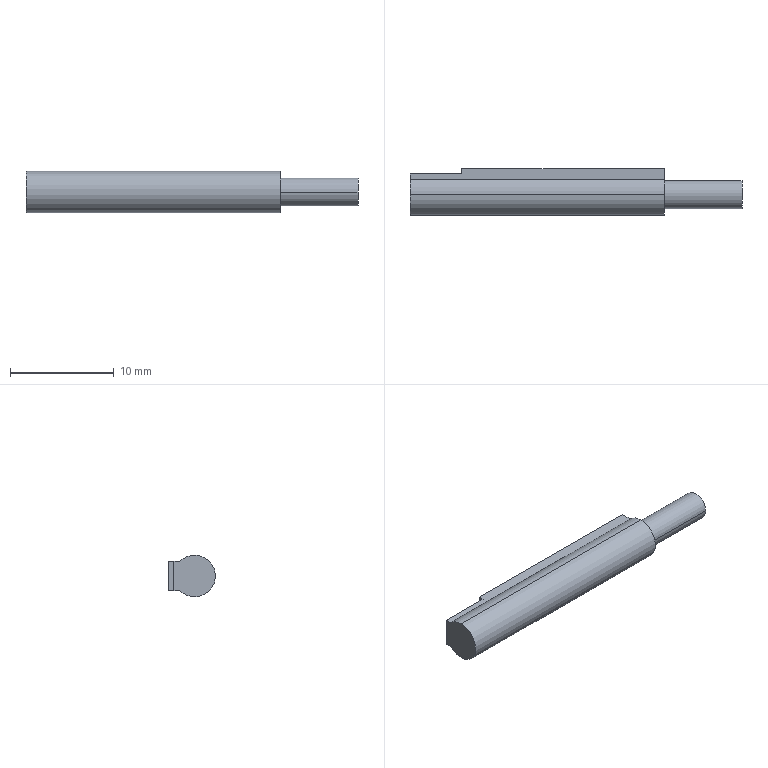Part | STEP file | 1105WWT3 | 1 solid | 16 faces | box 32 x 4.5 x 4 mm | volume 389.357 mm3 | plane 9 | cylinder 7 | commonest cylinder face diameters 4 x3 2.5 x2 2.7 x2
STEP:
#1=CARTESIAN_POINT('',(36.5,24.428,9.6));
#2=VERTEX_POINT('',#1);
#3=CARTESIAN_POINT('',(36.5,23.,9.));
#4=VERTEX_POINT('',#3);
#5=CARTESIAN_POINT('',(36.5,23.,11.));
#6=DIRECTION('',(-1.,0.,0.));
#7=DIRECTION('',(0.,0.,1.));
#8=AXIS2_PLACEMENT_3D('',#5,#6,#7);
#9=CIRCLE('',#8,2.);
#10=EDGE_CURVE('',#2,#4,#9,.T.);
#11=ORIENTED_EDGE('',*,*,#10,.T.);
#12=CARTESIAN_POINT('',(12.,23.,9.));
#13=VERTEX_POINT('',#12);
#14=CARTESIAN_POINT('',(12.,23.,9.));
#15=DIRECTION('',(-1.,0.,0.));
#16=VECTOR('',#15,1000.);
#17=LINE('',#14,#16);
#18=EDGE_CURVE('',#4,#13,#17,.T.);
#19=ORIENTED_EDGE('',*,*,#18,.T.);
#20=CARTESIAN_POINT('',(12.,24.428,9.6));
#21=VERTEX_POINT('',#20);
#22=CARTESIAN_POINT('',(12.,23.,11.));
#23=DIRECTION('',(1.,0.,0.));
#24=DIRECTION('',(0.,0.,1.));
#25=AXIS2_PLACEMENT_3D('',#22,#23,#24);
#26=CIRCLE('',#25,2.);
#27=EDGE_CURVE('',#13,#21,#26,.T.);
#28=ORIENTED_EDGE('',*,*,#27,.T.);
#29=CARTESIAN_POINT('',(12.,24.428,9.6));
#30=DIRECTION('',(1.,0.,0.));
#31=VECTOR('',#30,1000.);
#32=LINE('',#29,#31);
#33=EDGE_CURVE('',#21,#2,#32,.T.);
#34=ORIENTED_EDGE('',*,*,#33,.T.);
#35=EDGE_LOOP('',(#11,#19,#28,#34));
#36=FACE_OUTER_BOUND('',#35,.T.);
#37=CARTESIAN_POINT('',(12.,23.,11.));
#38=DIRECTION('',(-1.,0.,0.));
#39=DIRECTION('',(0.,0.,1.));
#40=AXIS2_PLACEMENT_3D('',#37,#38,#39);
#41=CYLINDRICAL_SURFACE('',#40,2.);
#42=ADVANCED_FACE('',(#36),#41,.T.);
#43=ORIENTED_EDGE('',*,*,#18,.F.);
#44=CARTESIAN_POINT('',(36.5,23.,13.));
#45=VERTEX_POINT('',#44);
#46=CARTESIAN_POINT('',(36.5,23.,11.));
#47=DIRECTION('',(-1.,0.,0.));
#48=DIRECTION('',(0.,0.,1.));
#49=AXIS2_PLACEMENT_3D('',#46,#47,#48);
#50=CIRCLE('',#49,2.);
#51=EDGE_CURVE('',#4,#45,#50,.T.);
#52=ORIENTED_EDGE('',*,*,#51,.T.);
#53=CARTESIAN_POINT('',(12.,23.,13.));
#54=VERTEX_POINT('',#53);
#55=CARTESIAN_POINT('',(12.,23.,13.));
#56=DIRECTION('',(-1.,0.,0.));
#57=VECTOR('',#56,1000.);
#58=LINE('',#55,#57);
#59=EDGE_CURVE('',#45,#54,#58,.T.);
#60=ORIENTED_EDGE('',*,*,#59,.T.);
#61=CARTESIAN_POINT('',(12.,23.,11.));
#62=DIRECTION('',(1.,0.,0.));
#63=DIRECTION('',(0.,0.,1.));
#64=AXIS2_PLACEMENT_3D('',#61,#62,#63);
#65=CIRCLE('',#64,2.);
#66=EDGE_CURVE('',#54,#13,#65,.T.);
#67=ORIENTED_EDGE('',*,*,#66,.T.);
#68=EDGE_LOOP('',(#43,#52,#60,#67));
#69=FACE_OUTER_BOUND('',#68,.T.);
#70=CARTESIAN_POINT('',(12.,23.,11.));
#71=DIRECTION('',(-1.,0.,0.));
#72=DIRECTION('',(0.,0.,1.));
#73=AXIS2_PLACEMENT_3D('',#70,#71,#72);
#74=CYLINDRICAL_SURFACE('',#73,2.);
#75=ADVANCED_FACE('',(#69),#74,.T.);
#76=CARTESIAN_POINT('',(36.5,21.65,11.));
#77=VERTEX_POINT('',#76);
#78=CARTESIAN_POINT('',(36.5,24.35,11.));
#79=VERTEX_POINT('',#78);
#80=CARTESIAN_POINT('',(36.5,23.,11.));
#81=DIRECTION('',(-1.,0.,0.));
#82=DIRECTION('',(0.,1.,0.));
#83=AXIS2_PLACEMENT_3D('',#80,#81,#82);
#84=CIRCLE('',#83,1.35);
#85=EDGE_CURVE('',#77,#79,#84,.T.);
#86=ORIENTED_EDGE('',*,*,#85,.F.);
#87=CARTESIAN_POINT('',(44.,21.65,11.));
#88=VERTEX_POINT('',#87);
#89=CARTESIAN_POINT('',(39.,21.65,11.));
#90=DIRECTION('',(1.,0.,0.));
#91=VECTOR('',#90,1000.);
#92=LINE('',#89,#91);
#93=EDGE_CURVE('',#77,#88,#92,.T.);
#94=ORIENTED_EDGE('',*,*,#93,.T.);
#95=CARTESIAN_POINT('',(44.,24.35,11.));
#96=VERTEX_POINT('',#95);
#97=CARTESIAN_POINT('',(44.,23.,11.));
#98=DIRECTION('',(-1.,0.,0.));
#99=DIRECTION('',(0.,1.,0.));
#100=AXIS2_PLACEMENT_3D('',#97,#98,#99);
#101=CIRCLE('',#100,1.35);
#102=EDGE_CURVE('',#88,#96,#101,.T.);
#103=ORIENTED_EDGE('',*,*,#102,.T.);
#104=CARTESIAN_POINT('',(39.,24.35,11.));
#105=DIRECTION('',(1.,0.,0.));
#106=VECTOR('',#105,1000.);
#107=LINE('',#104,#106);
#108=EDGE_CURVE('',#79,#96,#107,.T.);
#109=ORIENTED_EDGE('',*,*,#108,.F.);
#110=EDGE_LOOP('',(#86,#94,#103,#109));
#111=FACE_OUTER_BOUND('',#110,.T.);
#112=CARTESIAN_POINT('',(39.,23.,11.));
#113=DIRECTION('',(1.,0.,0.));
#114=DIRECTION('',(0.,1.,0.));
#115=AXIS2_PLACEMENT_3D('',#112,#113,#114);
#116=CYLINDRICAL_SURFACE('',#115,1.35);
#117=ADVANCED_FACE('',(#111),#116,.T.);
#118=CARTESIAN_POINT('',(14.,24.8,9.75));
#119=VERTEX_POINT('',#118);
#120=CARTESIAN_POINT('',(14.,24.8,12.25));
#121=VERTEX_POINT('',#120);
#122=CARTESIAN_POINT('',(14.,24.8,11.));
#123=DIRECTION('',(0.,1.,0.));
#124=DIRECTION('',(0.,0.,1.));
#125=AXIS2_PLACEMENT_3D('',#122,#123,#124);
#126=CIRCLE('',#125,1.25);
#127=EDGE_CURVE('',#119,#121,#126,.T.);
#128=ORIENTED_EDGE('',*,*,#127,.F.);
#129=CARTESIAN_POINT('',(14.,25.,9.75));
#130=VERTEX_POINT('',#129);
#131=CARTESIAN_POINT('',(14.,25.,9.75));
#132=DIRECTION('',(0.,1.,0.));
#133=VECTOR('',#132,1000.);
#134=LINE('',#131,#133);
#135=EDGE_CURVE('',#119,#130,#134,.T.);
#136=ORIENTED_EDGE('',*,*,#135,.T.);
#137=CARTESIAN_POINT('',(14.,25.,12.25));
#138=VERTEX_POINT('',#137);
#139=CARTESIAN_POINT('',(14.,25.,11.));
#140=DIRECTION('',(0.,1.,0.));
#141=DIRECTION('',(0.,0.,1.));
#142=AXIS2_PLACEMENT_3D('',#139,#140,#141);
#143=CIRCLE('',#142,1.25);
#144=EDGE_CURVE('',#130,#138,#143,.T.);
#145=ORIENTED_EDGE('',*,*,#144,.T.);
#146=CARTESIAN_POINT('',(14.,25.,12.25));
#147=DIRECTION('',(0.,1.,0.));
#148=VECTOR('',#147,1000.);
#149=LINE('',#146,#148);
#150=EDGE_CURVE('',#121,#138,#149,.T.);
#151=ORIENTED_EDGE('',*,*,#150,.F.);
#152=EDGE_LOOP('',(#128,#136,#145,#151));
#153=FACE_OUTER_BOUND('',#152,.T.);
#154=CARTESIAN_POINT('',(14.,25.,11.));
#155=DIRECTION('',(0.,1.,0.));
#156=DIRECTION('',(0.,0.,1.));
#157=AXIS2_PLACEMENT_3D('',#154,#155,#156);
#158=CYLINDRICAL_SURFACE('',#157,1.25);
#159=ADVANCED_FACE('',(#153),#158,.F.);
#160=ORIENTED_EDGE('',*,*,#59,.F.);
#161=CARTESIAN_POINT('',(36.5,24.428,12.4));
#162=VERTEX_POINT('',#161);
#163=CARTESIAN_POINT('',(36.5,23.,11.));
#164=DIRECTION('',(-1.,0.,0.));
#165=DIRECTION('',(0.,0.,1.));
#166=AXIS2_PLACEMENT_3D('',#163,#164,#165);
#167=CIRCLE('',#166,2.);
#168=EDGE_CURVE('',#45,#162,#167,.T.);
#169=ORIENTED_EDGE('',*,*,#168,.T.);
#170=CARTESIAN_POINT('',(12.,24.428,12.4));
#171=VERTEX_POINT('',#170);
#172=CARTESIAN_POINT('',(12.,24.428,12.4));
#173=DIRECTION('',(-1.,0.,0.));
#174=VECTOR('',#173,1000.);
#175=LINE('',#172,#174);
#176=EDGE_CURVE('',#162,#171,#175,.T.);
#177=ORIENTED_EDGE('',*,*,#176,.T.);
#178=CARTESIAN_POINT('',(12.,23.,11.));
#179=DIRECTION('',(1.,0.,0.));
#180=DIRECTION('',(0.,0.,1.));
#181=AXIS2_PLACEMENT_3D('',#178,#179,#180);
#182=CIRCLE('',#181,2.);
#183=EDGE_CURVE('',#171,#54,#182,.T.);
#184=ORIENTED_EDGE('',*,*,#183,.T.);
#185=EDGE_LOOP('',(#160,#169,#177,#184));
#186=FACE_OUTER_BOUND('',#185,.T.);
#187=CARTESIAN_POINT('',(12.,23.,11.));
#188=DIRECTION('',(-1.,0.,0.));
#189=DIRECTION('',(0.,0.,1.));
#190=AXIS2_PLACEMENT_3D('',#187,#188,#189);
#191=CYLINDRICAL_SURFACE('',#190,2.);
#192=ADVANCED_FACE('',(#186),#191,.T.);
#193=CARTESIAN_POINT('',(12.,25.,9.6));
#194=VERTEX_POINT('',#193);
#195=CARTESIAN_POINT('',(12.,25.5,9.6));
#196=DIRECTION('',(0.,1.,0.));
#197=VECTOR('',#196,1000.);
#198=LINE('',#195,#197);
#199=EDGE_CURVE('',#21,#194,#198,.T.);
#200=ORIENTED_EDGE('',*,*,#199,.F.);
#201=ORIENTED_EDGE('',*,*,#27,.F.);
#202=ORIENTED_EDGE('',*,*,#66,.F.);
#203=ORIENTED_EDGE('',*,*,#183,.F.);
#204=CARTESIAN_POINT('',(12.,25.,12.4));
#205=VERTEX_POINT('',#204);
#206=CARTESIAN_POINT('',(12.,23.,12.4));
#207=DIRECTION('',(0.,-1.,0.));
#208=VECTOR('',#207,1000.);
#209=LINE('',#206,#208);
#210=EDGE_CURVE('',#205,#171,#209,.T.);
#211=ORIENTED_EDGE('',*,*,#210,.F.);
#212=CARTESIAN_POINT('',(12.,25.,11.));
#213=DIRECTION('',(0.,0.,1.));
#214=VECTOR('',#213,1000.);
#215=LINE('',#212,#214);
#216=EDGE_CURVE('',#194,#205,#215,.T.);
#217=ORIENTED_EDGE('',*,*,#216,.F.);
#218=EDGE_LOOP('',(#200,#201,#202,#203,#211,#217));
#219=FACE_OUTER_BOUND('',#218,.T.);
#220=CARTESIAN_POINT('',(12.,23.,11.));
#221=DIRECTION('',(1.,0.,0.));
#222=DIRECTION('',(0.,0.,-1.));
#223=AXIS2_PLACEMENT_3D('',#220,#221,#222);
#224=PLANE('',#223);
#225=ADVANCED_FACE('',(#219),#224,.F.);
#226=CARTESIAN_POINT('',(36.5,25.5,12.4));
#227=VERTEX_POINT('',#226);
#228=CARTESIAN_POINT('',(36.5,24.428,12.4));
#229=DIRECTION('',(0.,1.,0.));
#230=VECTOR('',#229,1000.);
#231=LINE('',#228,#230);
#232=EDGE_CURVE('',#162,#227,#231,.T.);
#233=ORIENTED_EDGE('',*,*,#232,.T.);
#234=CARTESIAN_POINT('',(17.,25.5,12.4));
#235=VERTEX_POINT('',#234);
#236=CARTESIAN_POINT('',(12.,25.5,12.4));
#237=DIRECTION('',(-1.,0.,0.));
#238=VECTOR('',#237,1000.);
#239=LINE('',#236,#238);
#240=EDGE_CURVE('',#227,#235,#239,.T.);
#241=ORIENTED_EDGE('',*,*,#240,.T.);
#242=CARTESIAN_POINT('',(17.,25.,12.4));
#243=VERTEX_POINT('',#242);
#244=CARTESIAN_POINT('',(17.,23.,12.4));
#245=DIRECTION('',(0.,-1.,0.));
#246=VECTOR('',#245,1000.);
#247=LINE('',#244,#246);
#248=EDGE_CURVE('',#235,#243,#247,.T.);
#249=ORIENTED_EDGE('',*,*,#248,.T.);
#250=CARTESIAN_POINT('',(12.,25.,12.4));
#251=DIRECTION('',(-1.,0.,0.));
#252=VECTOR('',#251,1000.);
#253=LINE('',#250,#252);
#254=EDGE_CURVE('',#243,#205,#253,.T.);
#255=ORIENTED_EDGE('',*,*,#254,.T.);
#256=ORIENTED_EDGE('',*,*,#210,.T.);
#257=ORIENTED_EDGE('',*,*,#176,.F.);
#258=EDGE_LOOP('',(#233,#241,#249,#255,#256,#257));
#259=FACE_OUTER_BOUND('',#258,.T.);
#260=CARTESIAN_POINT('',(12.,24.428,12.4));
#261=DIRECTION('',(0.,0.,1.));
#262=DIRECTION('',(1.,0.,0.));
#263=AXIS2_PLACEMENT_3D('',#260,#261,#262);
#264=PLANE('',#263);
#265=ADVANCED_FACE('',(#259),#264,.T.);
#266=CARTESIAN_POINT('',(36.5,25.5,9.6));
#267=VERTEX_POINT('',#266);
#268=CARTESIAN_POINT('',(36.5,25.5,9.6));
#269=DIRECTION('',(0.,-1.,0.));
#270=VECTOR('',#269,1000.);
#271=LINE('',#268,#270);
#272=EDGE_CURVE('',#267,#2,#271,.T.);
#273=ORIENTED_EDGE('',*,*,#272,.F.);
#274=CARTESIAN_POINT('',(36.5,25.5,11.));
#275=DIRECTION('',(0.,0.,1.));
#276=VECTOR('',#275,1000.);
#277=LINE('',#274,#276);
#278=EDGE_CURVE('',#267,#227,#277,.T.);
#279=ORIENTED_EDGE('',*,*,#278,.T.);
#280=ORIENTED_EDGE('',*,*,#232,.F.);
#281=ORIENTED_EDGE('',*,*,#168,.F.);
#282=ORIENTED_EDGE('',*,*,#51,.F.);
#283=ORIENTED_EDGE('',*,*,#10,.F.);
#284=EDGE_LOOP('',(#273,#279,#280,#281,#282,#283));
#285=FACE_OUTER_BOUND('',#284,.T.);
#286=CARTESIAN_POINT('',(36.5,23.,11.));
#287=DIRECTION('',(-1.,0.,0.));
#288=DIRECTION('',(0.,1.,0.));
#289=AXIS2_PLACEMENT_3D('',#286,#287,#288);
#290=CIRCLE('',#289,1.35);
#291=EDGE_CURVE('',#79,#77,#290,.T.);
#292=ORIENTED_EDGE('',*,*,#291,.T.);
#293=ORIENTED_EDGE('',*,*,#85,.T.);
#294=EDGE_LOOP('',(#292,#293));
#295=FACE_BOUND('',#294,.T.);
#296=CARTESIAN_POINT('',(36.5,23.,11.));
#297=DIRECTION('',(1.,0.,0.));
#298=DIRECTION('',(0.,0.,-1.));
#299=AXIS2_PLACEMENT_3D('',#296,#297,#298);
#300=PLANE('',#299);
#301=ADVANCED_FACE('',(#285,#295),#300,.T.);
#302=CARTESIAN_POINT('',(17.,25.,9.6));
#303=VERTEX_POINT('',#302);
#304=CARTESIAN_POINT('',(12.,25.,9.6));
#305=DIRECTION('',(1.,0.,0.));
#306=VECTOR('',#305,1000.);
#307=LINE('',#304,#306);
#308=EDGE_CURVE('',#194,#303,#307,.T.);
#309=ORIENTED_EDGE('',*,*,#308,.F.);
#310=ORIENTED_EDGE('',*,*,#216,.T.);
#311=ORIENTED_EDGE('',*,*,#254,.F.);
#312=CARTESIAN_POINT('',(17.,25.,9.6));
#313=DIRECTION('',(0.,0.,1.));
#314=VECTOR('',#313,1000.);
#315=LINE('',#312,#314);
#316=EDGE_CURVE('',#303,#243,#315,.T.);
#317=ORIENTED_EDGE('',*,*,#316,.F.);
#318=EDGE_LOOP('',(#309,#310,#311,#317));
#319=FACE_OUTER_BOUND('',#318,.T.);
#320=CARTESIAN_POINT('',(14.,25.,11.));
#321=DIRECTION('',(0.,1.,0.));
#322=DIRECTION('',(0.,0.,1.));
#323=AXIS2_PLACEMENT_3D('',#320,#321,#322);
#324=CIRCLE('',#323,1.25);
#325=EDGE_CURVE('',#138,#130,#324,.T.);
#326=ORIENTED_EDGE('',*,*,#325,.F.);
#327=ORIENTED_EDGE('',*,*,#144,.F.);
#328=EDGE_LOOP('',(#326,#327));
#329=FACE_BOUND('',#328,.T.);
#330=CARTESIAN_POINT('',(12.,25.,9.6));
#331=DIRECTION('',(0.,-1.,0.));
#332=DIRECTION('',(0.,0.,-1.));
#333=AXIS2_PLACEMENT_3D('',#330,#331,#332);
#334=PLANE('',#333);
#335=ADVANCED_FACE('',(#319,#329),#334,.F.);
#336=ORIENTED_EDGE('',*,*,#278,.F.);
#337=CARTESIAN_POINT('',(17.,25.5,9.6));
#338=VERTEX_POINT('',#337);
#339=CARTESIAN_POINT('',(12.,25.5,9.6));
#340=DIRECTION('',(-1.,0.,0.));
#341=VECTOR('',#340,1000.);
#342=LINE('',#339,#341);
#343=EDGE_CURVE('',#267,#338,#342,.T.);
#344=ORIENTED_EDGE('',*,*,#343,.T.);
#345=CARTESIAN_POINT('',(17.,25.5,12.4));
#346=DIRECTION('',(0.,0.,1.));
#347=VECTOR('',#346,1000.);
#348=LINE('',#345,#347);
#349=EDGE_CURVE('',#338,#235,#348,.T.);
#350=ORIENTED_EDGE('',*,*,#349,.T.);
#351=ORIENTED_EDGE('',*,*,#240,.F.);
#352=EDGE_LOOP('',(#336,#344,#350,#351));
#353=FACE_OUTER_BOUND('',#352,.T.);
#354=CARTESIAN_POINT('',(12.,25.5,12.4));
#355=DIRECTION('',(0.,1.,0.));
#356=DIRECTION('',(0.,0.,1.));
#357=AXIS2_PLACEMENT_3D('',#354,#355,#356);
#358=PLANE('',#357);
#359=ADVANCED_FACE('',(#353),#358,.T.);
#360=ORIENTED_EDGE('',*,*,#93,.F.);
#361=ORIENTED_EDGE('',*,*,#291,.F.);
#362=ORIENTED_EDGE('',*,*,#108,.T.);
#363=CARTESIAN_POINT('',(44.,23.,11.));
#364=DIRECTION('',(-1.,0.,0.));
#365=DIRECTION('',(0.,1.,0.));
#366=AXIS2_PLACEMENT_3D('',#363,#364,#365);
#367=CIRCLE('',#366,1.35);
#368=EDGE_CURVE('',#96,#88,#367,.T.);
#369=ORIENTED_EDGE('',*,*,#368,.T.);
#370=EDGE_LOOP('',(#360,#361,#362,#369));
#371=FACE_OUTER_BOUND('',#370,.T.);
#372=CARTESIAN_POINT('',(39.,23.,11.));
#373=DIRECTION('',(1.,0.,0.));
#374=DIRECTION('',(0.,1.,0.));
#375=AXIS2_PLACEMENT_3D('',#372,#373,#374);
#376=CYLINDRICAL_SURFACE('',#375,1.35);
#377=ADVANCED_FACE('',(#371),#376,.T.);
#378=ORIENTED_EDGE('',*,*,#199,.T.);
#379=ORIENTED_EDGE('',*,*,#308,.T.);
#380=CARTESIAN_POINT('',(17.,25.5,9.6));
#381=DIRECTION('',(0.,1.,0.));
#382=VECTOR('',#381,1000.);
#383=LINE('',#380,#382);
#384=EDGE_CURVE('',#303,#338,#383,.T.);
#385=ORIENTED_EDGE('',*,*,#384,.T.);
#386=ORIENTED_EDGE('',*,*,#343,.F.);
#387=ORIENTED_EDGE('',*,*,#272,.T.);
#388=ORIENTED_EDGE('',*,*,#33,.F.);
#389=EDGE_LOOP('',(#378,#379,#385,#386,#387,#388));
#390=FACE_OUTER_BOUND('',#389,.T.);
#391=CARTESIAN_POINT('',(12.,25.5,9.6));
#392=DIRECTION('',(0.,0.,-1.));
#393=DIRECTION('',(-1.,0.,0.));
#394=AXIS2_PLACEMENT_3D('',#391,#392,#393);
#395=PLANE('',#394);
#396=ADVANCED_FACE('',(#390),#395,.T.);
#397=ORIENTED_EDGE('',*,*,#384,.F.);
#398=ORIENTED_EDGE('',*,*,#316,.T.);
#399=ORIENTED_EDGE('',*,*,#248,.F.);
#400=ORIENTED_EDGE('',*,*,#349,.F.);
#401=EDGE_LOOP('',(#397,#398,#399,#400));
#402=FACE_OUTER_BOUND('',#401,.T.);
#403=CARTESIAN_POINT('',(17.,23.,11.));
#404=DIRECTION('',(1.,0.,0.));
#405=DIRECTION('',(0.,0.,-1.));
#406=AXIS2_PLACEMENT_3D('',#403,#404,#405);
#407=PLANE('',#406);
#408=ADVANCED_FACE('',(#402),#407,.F.);
#409=ORIENTED_EDGE('',*,*,#135,.F.);
#410=CARTESIAN_POINT('',(14.,24.8,11.));
#411=DIRECTION('',(0.,1.,0.));
#412=DIRECTION('',(0.,0.,1.));
#413=AXIS2_PLACEMENT_3D('',#410,#411,#412);
#414=CIRCLE('',#413,1.25);
#415=EDGE_CURVE('',#121,#119,#414,.T.);
#416=ORIENTED_EDGE('',*,*,#415,.F.);
#417=ORIENTED_EDGE('',*,*,#150,.T.);
#418=ORIENTED_EDGE('',*,*,#325,.T.);
#419=EDGE_LOOP('',(#409,#416,#417,#418));
#420=FACE_OUTER_BOUND('',#419,.T.);
#421=CARTESIAN_POINT('',(14.,25.,11.));
#422=DIRECTION('',(0.,1.,0.));
#423=DIRECTION('',(0.,0.,1.));
#424=AXIS2_PLACEMENT_3D('',#421,#422,#423);
#425=CYLINDRICAL_SURFACE('',#424,1.25);
#426=ADVANCED_FACE('',(#420),#425,.F.);
#427=ORIENTED_EDGE('',*,*,#368,.F.);
#428=ORIENTED_EDGE('',*,*,#102,.F.);
#429=EDGE_LOOP('',(#427,#428));
#430=FACE_OUTER_BOUND('',#429,.T.);
#431=CARTESIAN_POINT('',(44.,23.675,11.));
#432=DIRECTION('',(1.,0.,0.));
#433=DIRECTION('',(0.,0.,-1.));
#434=AXIS2_PLACEMENT_3D('',#431,#432,#433);
#435=PLANE('',#434);
#436=ADVANCED_FACE('',(#430),#435,.T.);
#437=ORIENTED_EDGE('',*,*,#415,.T.);
#438=ORIENTED_EDGE('',*,*,#127,.T.);
#439=EDGE_LOOP('',(#437,#438));
#440=FACE_OUTER_BOUND('',#439,.T.);
#441=CARTESIAN_POINT('',(12.,24.8,11.));
#442=DIRECTION('',(0.,1.,0.));
#443=DIRECTION('',(0.,0.,1.));
#444=AXIS2_PLACEMENT_3D('',#441,#442,#443);
#445=PLANE('',#444);
#446=ADVANCED_FACE('',(#440),#445,.T.);
#447=CLOSED_SHELL('',(#42,#75,#117,#159,#192,#225,#265,#301,#335,#359,#377,#396,#408,#426,#436,#446));
#448=MANIFOLD_SOLID_BREP('',#447);
#449=CARTESIAN_POINT('',(0.,0.,0.));
#450=DIRECTION('',(0.,0.,1.));
#451=DIRECTION('',(1.,0.,0.));
#452=AXIS2_PLACEMENT_3D('',#449,#450,#451);
#453=(LENGTH_UNIT()NAMED_UNIT(*)SI_UNIT(.MILLI.,.METRE.));
#454=UNCERTAINTY_MEASURE_WITH_UNIT(LENGTH_MEASURE(0.00001),#453,'','');
#455=(NAMED_UNIT(*)PLANE_ANGLE_UNIT()SI_UNIT($,.RADIAN.));
#456=(NAMED_UNIT(*)SI_UNIT($,.STERADIAN.)SOLID_ANGLE_UNIT());
#457=(GEOMETRIC_REPRESENTATION_CONTEXT(3)GLOBAL_UNCERTAINTY_ASSIGNED_CONTEXT((#454))GLOBAL_UNIT_ASSIGNED_CONTEXT((#453,#455,#456))REPRESENTATION_CONTEXT('',''));
#458=ADVANCED_BREP_SHAPE_REPRESENTATION('',(#448,#452),#457);